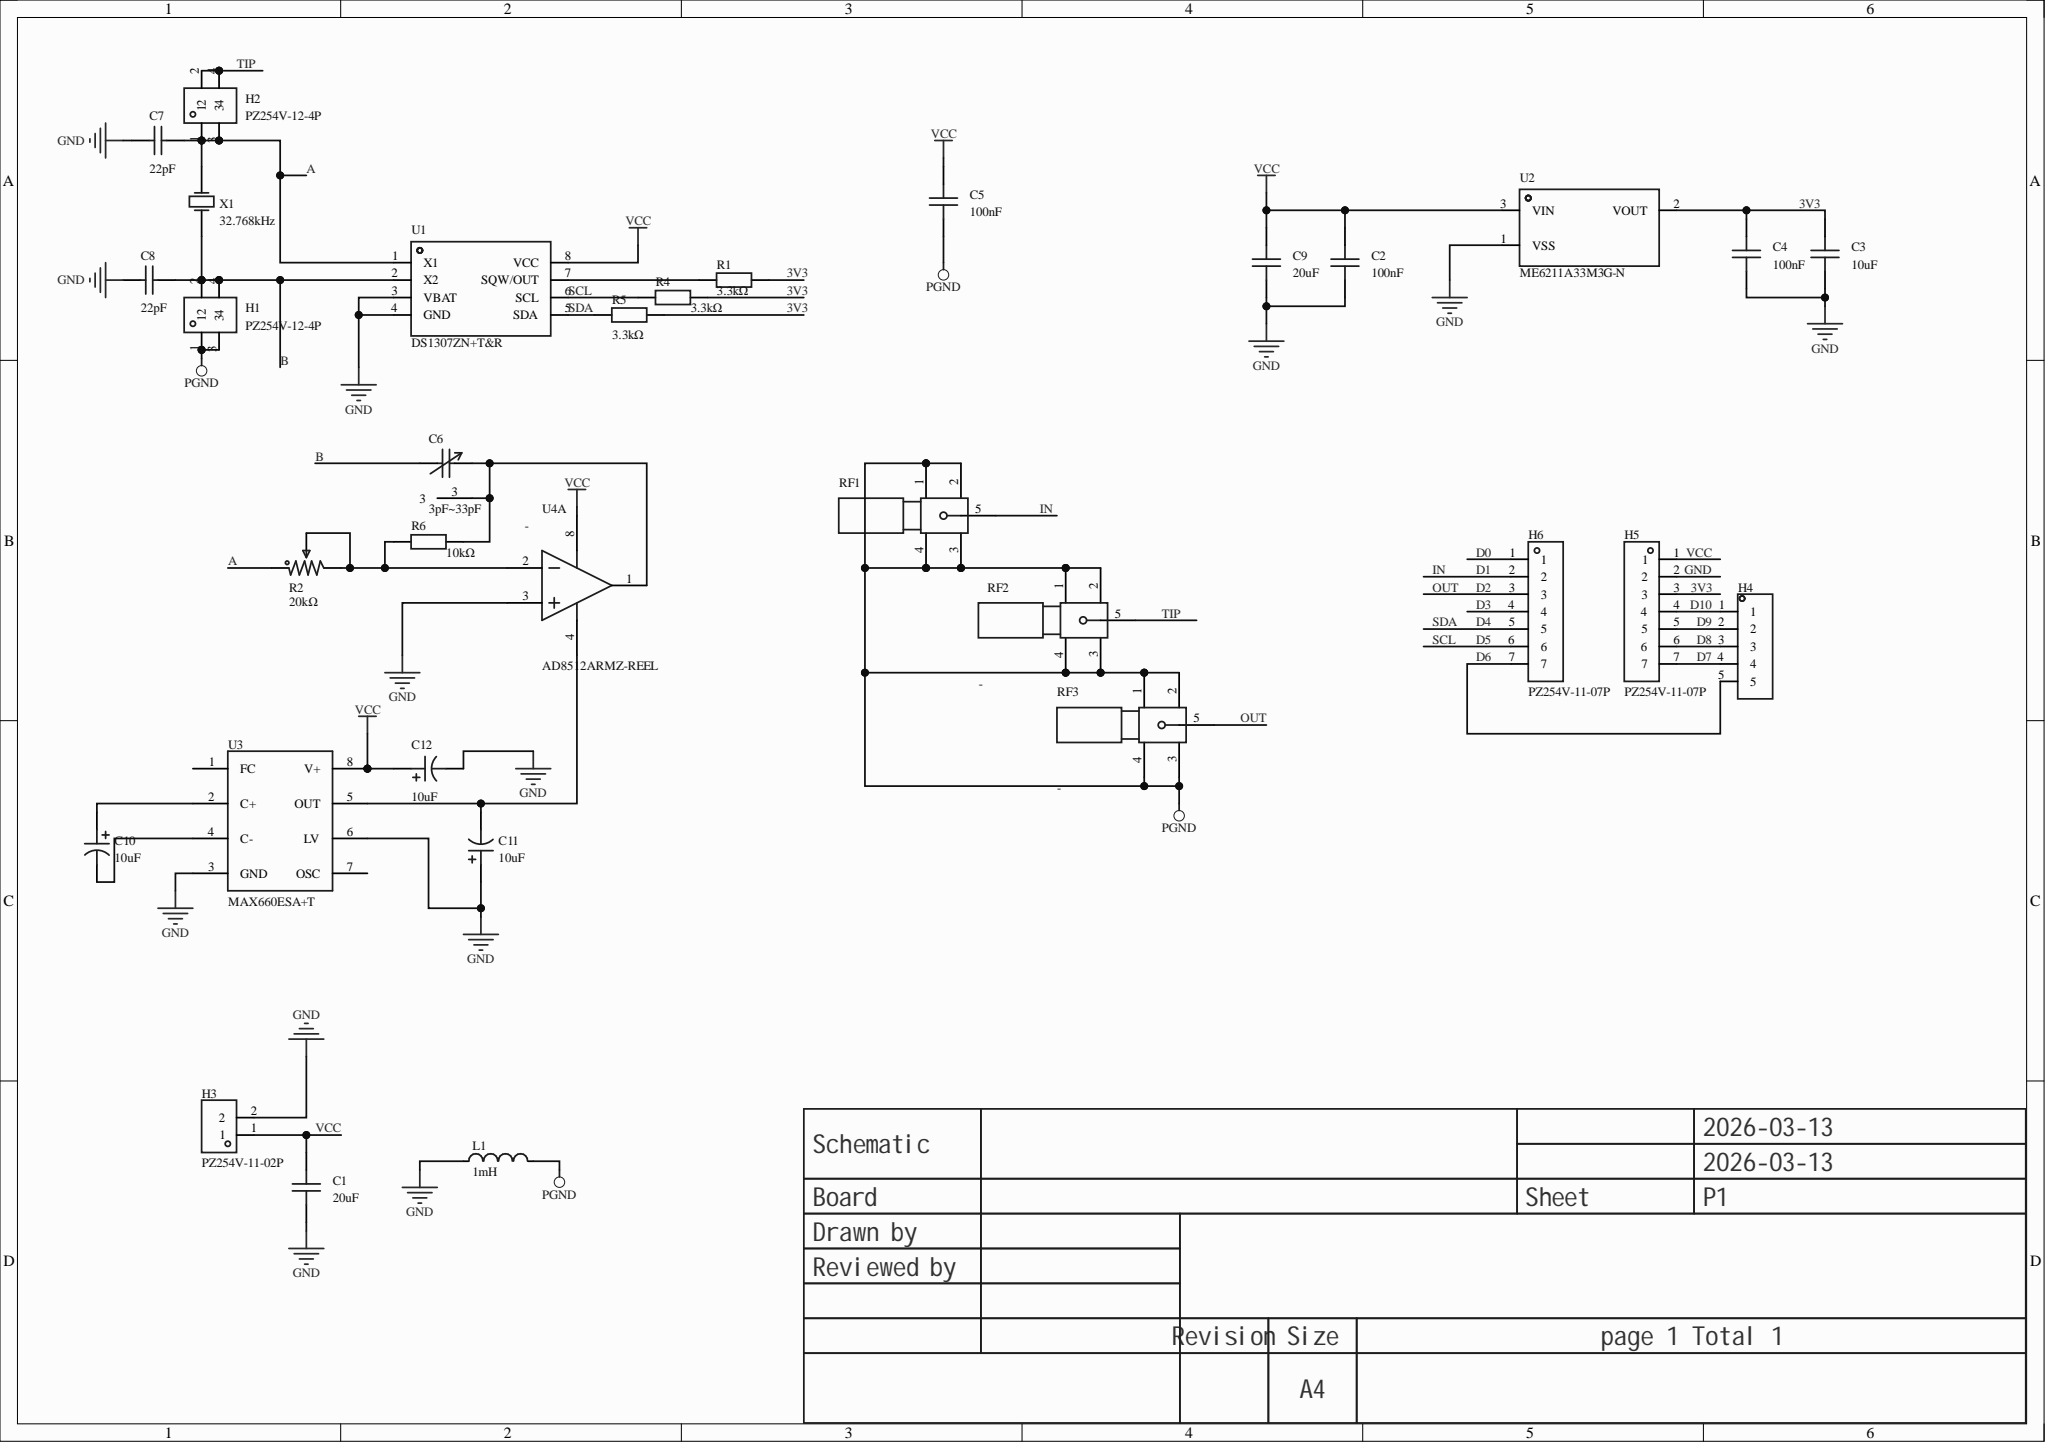Circuit board | Altium Designer | 32 parts | 22 nets
Bill of materials:
Comment,Description,Designator,Footprint,LibRef,Quantity
"20uF","Capacitance:20uF;Tolerance:±20%;Rated voltage:16V;Temperature coefficient:X5R;","C1, C9","CAP-SMD_L1.8-W1.0","GRMJN7R61C206ME05D","2"
"100nF","Capacitance:100nF;Tolerance:±10%;Rated voltage:50V;Temperature coefficient:X7R;","C2, C4, C5","C0603","CGA0603X7R104K500JT","3"
"10uF","Capacitance:10uF;Tolerance:±10%;Rated voltage:10V;Temperature coefficient:X5R;","C3","C0603","CGA0603X5R106K100JT","1"
"3pF~33pF","Capacitance:3pF~33pF;Rated voltage:250V;Charge:-;","C6","CAP-ADJ-TH_3P-BD7.6_BFC280811339","BFC280811339","1"
"22pF","Capacitance:22pF;Tolerance:±5%;Rated voltage:50V;Temperature coefficient:C0G;","C7, C8","C0603","CL10C220JB8NNNC","2"
"10uF","Capacitance:10uF;Tolerance:±20%;Rated voltage:50V;Ripple current:18mA@120Hz;","C10, C11, C12","CAP-SMD_BD5.0-L5.3-W5.3-LS6.0-FD","JVJ50v10M5x5","3"
"PZ254V-12-4P","Pin structure:2x2P;Pitch:2.54mm;Row spacing:2.54mm;Round/square pin:Square pin;Mounting:Through-hole;Rows:Double row;Total pins:4P;Rated current:-;Rated voltage:-;Mating pin length:6mm;Plastic height:2.5mm;Tail length:3mm;Contact material:Brass;Contact plating:-;Operating temperature:-40℃~+105℃;Color:Black;","H1, H2","HDR-TH_4P-P2.54-V-M-R2-C2-S2.54","PZ254V-12-4P","2"
"PZ254V-11-02P","Pin structure:1x2P;Pitch:2.54mm;Row spacing:-;Round/square pin:Square pin;Mounting:Through-hole;Rows:Single row;Total pins:2P;Rated current:-;Rated voltage:-;Mating pin length:6mm;Plastic height:2.5mm;Tail length:3mm;Contact material:Brass;Contact plating:-;Operating temperature:-40℃~+105℃;Color:Black;","H3","HDR-TH_2P-P2.54-V-M","PZ254V-11-02P","1"
"","","H4","HDR-TH_5P-P2.54-V-M","HDR-M_2.54_1x5P","1"
"PZ254V-11-07P","Pin structure:1x7P;Pitch:2.54mm;Row spacing:-;Round/square pin:Square pin;Mounting:Through-hole;Rows:Single row;Total pins:7P;Rated current:-;Rated voltage:-;Mating pin length:6mm;Plastic height:2.5mm;Tail length:3mm;Contact material:Brass;Contact plating:-;Operating temperature:-40℃~+105℃;Color:Black;","H5, H6","HDR-TH_7P-P2.54-V-M","PZ254V-11-07P","2"
"1mH","Inductance:1mH;Tolerance:±20%;Rated current:500mA;Type:I-shaped inductor;","L1","IND-TH_BD8.5-P5.00-D0.6","SLP0810R-102MTT","1"
"3.3kΩ","Resistor type:Thick film resistor;Resistance:3.3kΩ;Tolerance:±1%;Power:100mW;Working voltage:75V;Temperature coefficient:±100ppm/?;","R1, R4, R5","R0603","0603WAF3301T5E","3"
"20kΩ","Resistance:10kΩ;Tolerance:±10%;Power:500mW;Temperature coefficient:±250ppm/?;","R2","RES-ADJ-TH_3362P","3362P-1-103_C48997914","1"
"10kΩ","Resistor type:Thick film resistor;Resistance:3.3kΩ;Tolerance:±1%;Power:100mW;Working voltage:75V;Temperature coefficient:±100ppm/?;","R6","R0603","0603WAF3301T5E","1"
"-","Connector type:Board mount;Interface type:Jack;Port count:1;Interface diameter:6.2mm;Interface length/height:8mm;Frequency:-;RF series:SMA;Impedance:-;Style:Straight pin;Operating temperature:-;","RF1, RF2, RF3","SMA-TH_KH-SMA-KE-Z","KH-SMA-KE-Z","3"
"DS1307ZN+T&R","Interface type:I2C;","U1","SOP-8_L4.9-W3.9-P1.27-LS6.0-BL","DS1307ZN+T&R","1"
"ME6211A33M3G-N","Output type:Fixed;Working voltage:6V;Output voltage:3.3V;Output current:500mA;Power supply rejection ratio (PSRR):70dB@(1kHz);Output polarity:Positive;","U2","SOT-23-3_L2.9-W1.6-P1.90-LS2.8-BR","ME6211A33M3G-N","1"
"MAX660ESA+T","CMOS single-chip voltage converter; converts input voltage by inversion or doubling","U3","SOIC-8_L5.0-W4.0-P1.27-LS6.0-BL","MAX660ESA+T","1"
"AD8512ARMZ-REEL","Amplifier count:Dual;Gain bandwidth product (GBP):8MHz;Input bias current (Ib):25pA;Input offset voltage (Vos):80uV;Slew rate (SR):20V/us;Rail-to-rail:-;","U4","MSOP-8_L3.0-W3.0-P0.65-LS5.0-TL","AD8512ARMZ-REEL","1"
"32.768kHz","Crystal type:Through-hole crystal;Frequency:32.768kHz;Frequency deviation at room temperature:±10ppm;Load capacitance:12.5pF;Frequency stability:±20ppm;","X1","OSC-TH_BD3.1-P0.8-D0.3","X308032768KGB2SC","1"
Netlist (Protel format):
[
C1
CAP-SMD_L1.8-W1.0
20uF



]
[
C2
C0603
100nF



]
[
C3
C0603
10uF



]
[
C4
C0603
100nF



]
[
C5
C0603
100nF



]
[
C6
CAP-ADJ-TH_3P-BD7.6_BFC280811339
3pF~33pF



]
[
C7
C0603
22pF



]
[
C8
C0603
22pF



]
[
C9
CAP-SMD_L1.8-W1.0
20uF



]
[
C10
CAP-SMD_BD5.0-L5.3-W5.3-LS6.0-FD
10uF



]
[
C11
CAP-SMD_BD5.0-L5.3-W5.3-LS6.0-FD
10uF



]
[
C12
CAP-SMD_BD5.0-L5.3-W5.3-LS6.0-FD
10uF



]
[
H1
HDR-TH_4P-P2.54-V-M-R2-C2-S2.54
PZ254V-12-4P



]
[
H2
HDR-TH_4P-P2.54-V-M-R2-C2-S2.54
PZ254V-12-4P



]
[
H3
HDR-TH_2P-P2.54-V-M
PZ254V-11-02P



]
[
H4
HDR-TH_5P-P2.54-V-M




]
[
H5
HDR-TH_7P-P2.54-V-M
PZ254V-11-07P



]
[
H6
HDR-TH_7P-P2.54-V-M
PZ254V-11-07P



]
[
L1
IND-TH_BD8.5-P5.00-D0.6
1mH



]
[
R1
R0603
3.3kΩ



]
[
R2
RES-ADJ-TH_3362P
20kΩ



]
[
R4
R0603
3.3kΩ



]
[
R5
R0603
3.3kΩ



]
[
R6
R0603
10kΩ



]
[
RF1
SMA-TH_KH-SMA-KE-Z
-



]
[
RF2
SMA-TH_KH-SMA-KE-Z
-



]
[
RF3
SMA-TH_KH-SMA-KE-Z
-



]
[
U1
SOP-8_L4.9-W3.9-P1.27-LS6.0-BL
DS1307ZN+T&R



]
[
U2
SOT-23-3_L2.9-W1.6-P1.90-LS2.8-BR
ME6211A33M3G-N



]
[
U3
SOIC-8_L5.0-W4.0-P1.27-LS6.0-BL
MAX660ESA+T



]
[
U4
MSOP-8_L3.0-W3.0-P0.65-LS5.0-TL
AD8512ARMZ-REEL



]
[
X1
OSC-TH_BD3.1-P0.8-D0.3
32.768kHz



]
(
VCC
C1-2
C2-2
C5-2
C9-2
C12-1
H3-1
H5-1
U1-8
U2-3
U3-8
U4-8
)
(
TIP
H2-2
H2-4
RF2-5
)
(
PGND
C5-1
H1-1
H1-3
L1-2
RF1-1
RF1-2
RF1-3
RF1-4
RF2-1
RF2-2
RF2-3
RF2-4
RF3-1
RF3-2
RF3-3
RF3-4
)
(
NetR2_2
R2-2
R2-3
R6-2
U4-2
)
(
NetR1_1
R1-1
U1-7
)
(
NetC11_2
C11-2
U3-5
U4-4
)
(
NetC10_2
C10-2
U3-4
)
(
NetC10_1
C10-1
U3-2
)
(
NetC6_2
C6-2
C6-3
R6-1
U4-1
)
(
GND
C1-1
C2-1
C3-1
C4-1
C7-2
C8-2
C9-1
C11-1
C12-2
H3-2
H5-2
L1-1
U1-3
U1-4
U2-1
U3-3
U3-6
U4-3
)
(
D10
H4-1
H5-4
)
(
D9
H4-2
H5-5
)
(
D8
H4-3
H5-6
)
(
D7
H4-4
H5-7
)
(
D6
H4-5
H6-7
)
(
D5
H6-6
R4-2
U1-6
)
(
D4
H6-5
R5-2
U1-5
)
(
D2
H6-3
RF3-5
)
(
D1
H6-2
RF1-5
)
(
B
C6-1
C8-1
H1-2
H1-4
U1-2
X1-1
)
(
A
C7-1
H2-1
H2-3
R2-1
U1-1
X1-2
)
(
3V3
C3-2
C4-2
H5-3
R1-2
R4-1
R5-1
U2-2
)